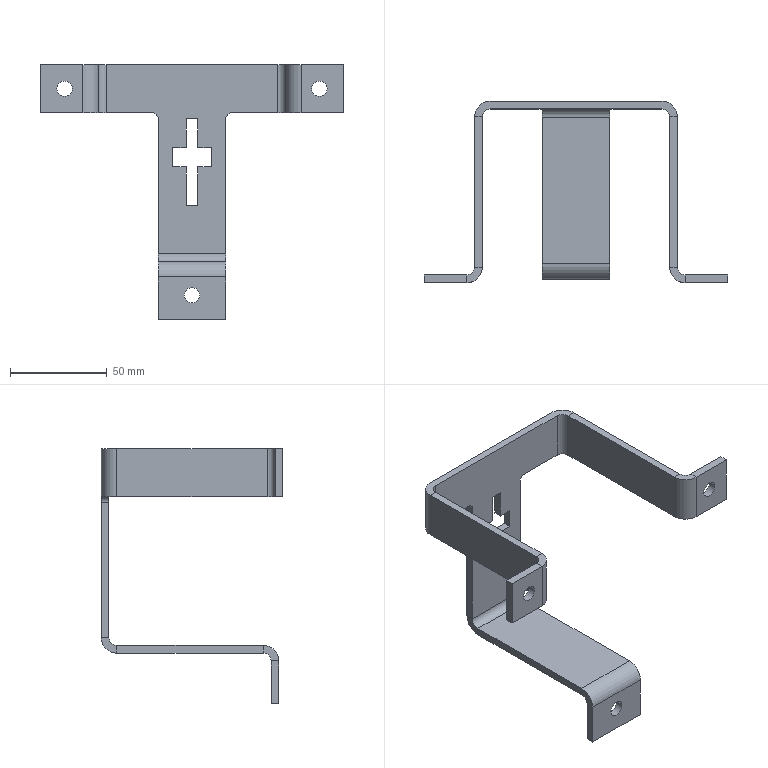Part | STEP file | 64562878 | 1 solid | 76 faces | box 157 x 94 x 132 mm | volume 57021 mm3 | plane 56 | cylinder 20 | commonest cylinder face diameters 8 x12 16 x6 6 x2